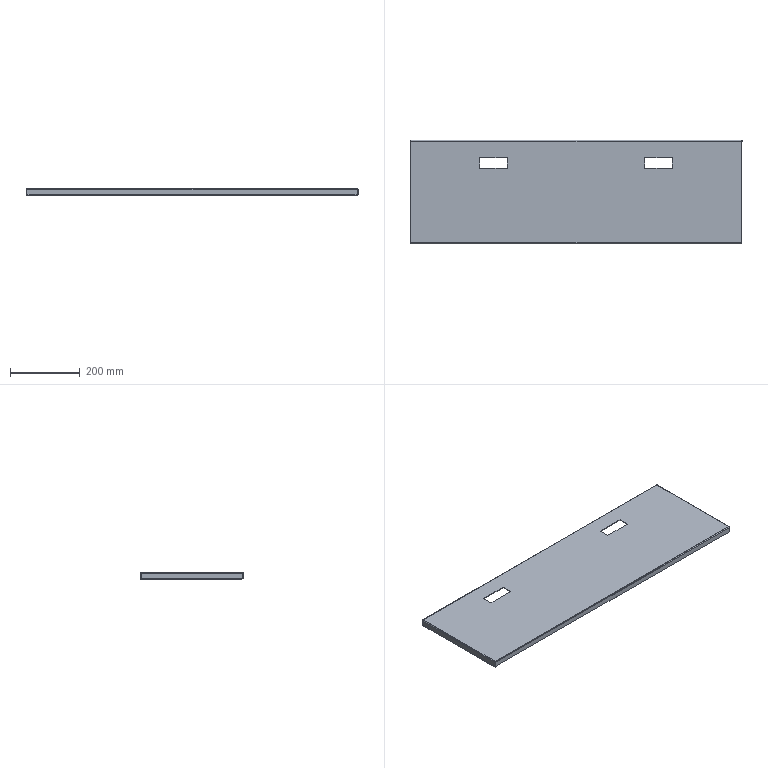Part | STEP file | 400v80 Rear Door Lower | 1 solid | 84 faces | box 955 x 297 x 20 mm | volume 675608 mm3 | plane 62 | cylinder 14 | spline 8 | commonest cylinder face diameters 1 x7 5 x7